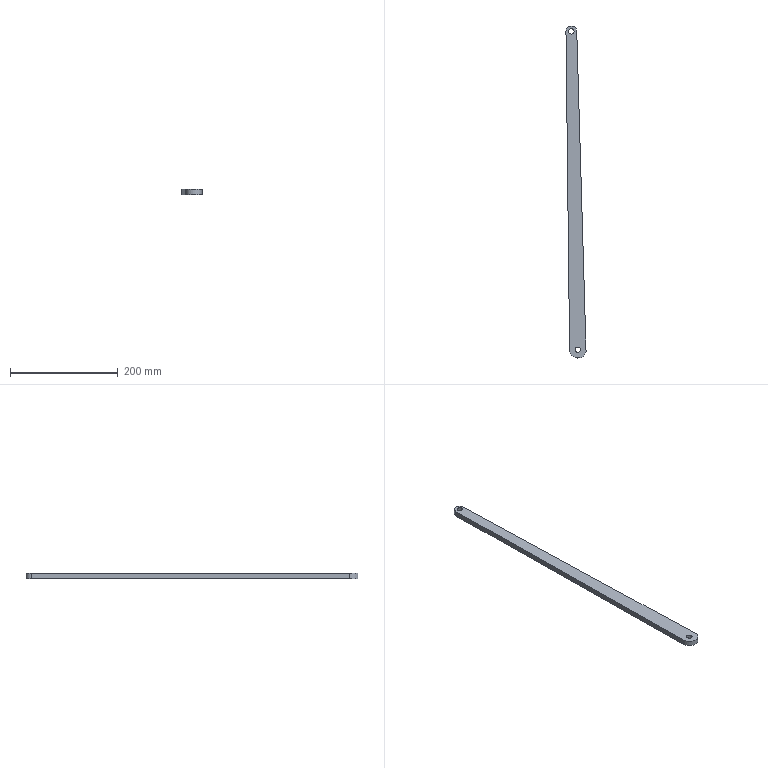Part | SolidWorks | features Extrusion 1 | 1 solid | 10 faces | box 37.197 x 615.099 x 10 mm | volume 152379 mm3 | cylinder 6 | plane 4 | commonest cylinder face diameters 10 x4 20 x1 30.679 x1
STEP:
#1=CARTESIAN_POINT('',(-4.803,1272.712,10.));
#2=VERTEX_POINT('',#1);
#3=CARTESIAN_POINT('',(5.197,1272.712,10.));
#4=VERTEX_POINT('',#3);
#5=CARTESIAN_POINT('',(0.1973,1272.712,10.));
#6=DIRECTION('',(0.,0.,1.));
#7=DIRECTION('',(1.,0.,0.));
#8=AXIS2_PLACEMENT_3D('',#5,#6,#7);
#9=CIRCLE('',#8,5.);
#10=EDGE_CURVE('',#2,#4,#9,.T.);
#11=ORIENTED_EDGE('',*,*,#10,.T.);
#12=CARTESIAN_POINT('',(5.197,1272.712,0.));
#13=VERTEX_POINT('',#12);
#14=CARTESIAN_POINT('',(5.197,1272.712,10.));
#15=DIRECTION('',(0.,0.,-1.));
#16=VECTOR('',#15,1000.);
#17=LINE('',#14,#16);
#18=EDGE_CURVE('',#4,#13,#17,.T.);
#19=ORIENTED_EDGE('',*,*,#18,.T.);
#20=CARTESIAN_POINT('',(-4.803,1272.712,0.));
#21=VERTEX_POINT('',#20);
#22=CARTESIAN_POINT('',(0.1973,1272.712,0.));
#23=DIRECTION('',(0.,0.,1.));
#24=DIRECTION('',(1.,0.,0.));
#25=AXIS2_PLACEMENT_3D('',#22,#23,#24);
#26=CIRCLE('',#25,5.);
#27=EDGE_CURVE('',#21,#13,#26,.T.);
#28=ORIENTED_EDGE('',*,*,#27,.F.);
#29=CARTESIAN_POINT('',(-4.803,1272.712,10.));
#30=DIRECTION('',(0.,0.,-1.));
#31=VECTOR('',#30,1000.);
#32=LINE('',#29,#31);
#33=EDGE_CURVE('',#2,#21,#32,.T.);
#34=ORIENTED_EDGE('',*,*,#33,.F.);
#35=EDGE_LOOP('',(#11,#19,#28,#34));
#36=FACE_OUTER_BOUND('',#35,.T.);
#37=CARTESIAN_POINT('',(0.1973,1272.712,10.));
#38=DIRECTION('',(0.,0.,-1.));
#39=DIRECTION('',(-1.,0.,0.));
#40=AXIS2_PLACEMENT_3D('',#37,#38,#39);
#41=CYLINDRICAL_SURFACE('',#40,5.);
#42=ADVANCED_FACE('',(#36),#41,.F.);
#43=CARTESIAN_POINT('',(7.243,682.953,10.));
#44=VERTEX_POINT('',#43);
#45=CARTESIAN_POINT('',(17.243,682.953,10.));
#46=VERTEX_POINT('',#45);
#47=CARTESIAN_POINT('',(12.243,682.953,10.));
#48=DIRECTION('',(0.,0.,1.));
#49=DIRECTION('',(1.,0.,0.));
#50=AXIS2_PLACEMENT_3D('',#47,#48,#49);
#51=CIRCLE('',#50,5.);
#52=EDGE_CURVE('',#44,#46,#51,.T.);
#53=ORIENTED_EDGE('',*,*,#52,.T.);
#54=CARTESIAN_POINT('',(17.243,682.953,0.));
#55=VERTEX_POINT('',#54);
#56=CARTESIAN_POINT('',(17.243,682.953,10.));
#57=DIRECTION('',(0.,0.,-1.));
#58=VECTOR('',#57,1000.);
#59=LINE('',#56,#58);
#60=EDGE_CURVE('',#46,#55,#59,.T.);
#61=ORIENTED_EDGE('',*,*,#60,.T.);
#62=CARTESIAN_POINT('',(7.243,682.953,0.));
#63=VERTEX_POINT('',#62);
#64=CARTESIAN_POINT('',(12.243,682.953,0.));
#65=DIRECTION('',(0.,0.,1.));
#66=DIRECTION('',(1.,0.,0.));
#67=AXIS2_PLACEMENT_3D('',#64,#65,#66);
#68=CIRCLE('',#67,5.);
#69=EDGE_CURVE('',#63,#55,#68,.T.);
#70=ORIENTED_EDGE('',*,*,#69,.F.);
#71=CARTESIAN_POINT('',(7.243,682.953,10.));
#72=DIRECTION('',(0.,0.,-1.));
#73=VECTOR('',#72,1000.);
#74=LINE('',#71,#73);
#75=EDGE_CURVE('',#44,#63,#74,.T.);
#76=ORIENTED_EDGE('',*,*,#75,.F.);
#77=EDGE_LOOP('',(#53,#61,#70,#76));
#78=FACE_OUTER_BOUND('',#77,.T.);
#79=CARTESIAN_POINT('',(12.243,682.953,10.));
#80=DIRECTION('',(0.,0.,-1.));
#81=DIRECTION('',(-1.,0.,0.));
#82=AXIS2_PLACEMENT_3D('',#79,#80,#81);
#83=CYLINDRICAL_SURFACE('',#82,5.);
#84=ADVANCED_FACE('',(#78),#83,.F.);
#85=CARTESIAN_POINT('',(-3.096,682.778,0.));
#86=VERTEX_POINT('',#85);
#87=CARTESIAN_POINT('',(-9.803,1272.712,0.));
#88=VERTEX_POINT('',#87);
#89=CARTESIAN_POINT('',(4.666,0.05305,0.));
#90=DIRECTION('',(-0.01137,0.9999,0.));
#91=VECTOR('',#90,1000.);
#92=LINE('',#89,#91);
#93=EDGE_CURVE('',#86,#88,#92,.T.);
#94=ORIENTED_EDGE('',*,*,#93,.F.);
#95=CARTESIAN_POINT('',(-3.096,682.778,10.));
#96=VERTEX_POINT('',#95);
#97=CARTESIAN_POINT('',(-3.096,682.778,10.));
#98=DIRECTION('',(0.,0.,-1.));
#99=VECTOR('',#98,1000.);
#100=LINE('',#97,#99);
#101=EDGE_CURVE('',#96,#86,#100,.T.);
#102=ORIENTED_EDGE('',*,*,#101,.F.);
#103=CARTESIAN_POINT('',(-9.803,1272.712,10.));
#104=VERTEX_POINT('',#103);
#105=CARTESIAN_POINT('',(4.666,0.05305,10.));
#106=DIRECTION('',(-0.01137,0.9999,0.));
#107=VECTOR('',#106,1000.);
#108=LINE('',#105,#107);
#109=EDGE_CURVE('',#96,#104,#108,.T.);
#110=ORIENTED_EDGE('',*,*,#109,.T.);
#111=CARTESIAN_POINT('',(-9.803,1272.712,10.));
#112=DIRECTION('',(0.,0.,-1.));
#113=VECTOR('',#112,1000.);
#114=LINE('',#111,#113);
#115=EDGE_CURVE('',#104,#88,#114,.T.);
#116=ORIENTED_EDGE('',*,*,#115,.T.);
#117=EDGE_LOOP('',(#94,#102,#110,#116));
#118=FACE_OUTER_BOUND('',#117,.T.);
#119=CARTESIAN_POINT('',(4.666,0.05305,10.));
#120=DIRECTION('',(-0.9999,-0.01137,0.));
#121=DIRECTION('',(0.01137,-0.9999,0.));
#122=AXIS2_PLACEMENT_3D('',#119,#120,#121);
#123=PLANE('',#122);
#124=ADVANCED_FACE('',(#118),#123,.T.);
#125=CARTESIAN_POINT('',(27.395,680.56,0.));
#126=VERTEX_POINT('',#125);
#127=CARTESIAN_POINT('',(12.243,682.953,0.));
#128=DIRECTION('',(0.,0.,1.));
#129=DIRECTION('',(1.,0.,0.));
#130=AXIS2_PLACEMENT_3D('',#127,#128,#129);
#131=CIRCLE('',#130,15.34);
#132=EDGE_CURVE('',#86,#126,#131,.T.);
#133=ORIENTED_EDGE('',*,*,#132,.T.);
#134=CARTESIAN_POINT('',(27.395,680.56,10.));
#135=VERTEX_POINT('',#134);
#136=CARTESIAN_POINT('',(27.395,680.56,10.));
#137=DIRECTION('',(0.,0.,-1.));
#138=VECTOR('',#137,1000.);
#139=LINE('',#136,#138);
#140=EDGE_CURVE('',#135,#126,#139,.T.);
#141=ORIENTED_EDGE('',*,*,#140,.F.);
#142=CARTESIAN_POINT('',(12.243,682.953,10.));
#143=DIRECTION('',(0.,0.,1.));
#144=DIRECTION('',(1.,0.,0.));
#145=AXIS2_PLACEMENT_3D('',#142,#143,#144);
#146=CIRCLE('',#145,15.34);
#147=EDGE_CURVE('',#96,#135,#146,.T.);
#148=ORIENTED_EDGE('',*,*,#147,.F.);
#149=ORIENTED_EDGE('',*,*,#101,.T.);
#150=EDGE_LOOP('',(#133,#141,#148,#149));
#151=FACE_OUTER_BOUND('',#150,.T.);
#152=CARTESIAN_POINT('',(12.243,682.953,10.));
#153=DIRECTION('',(0.,0.,-1.));
#154=DIRECTION('',(-1.,0.,0.));
#155=AXIS2_PLACEMENT_3D('',#152,#153,#154);
#156=CYLINDRICAL_SURFACE('',#155,15.34);
#157=ADVANCED_FACE('',(#151),#156,.T.);
#158=CARTESIAN_POINT('',(10.197,1272.712,0.));
#159=VERTEX_POINT('',#158);
#160=CARTESIAN_POINT('',(47.12,1.368,0.));
#161=DIRECTION('',(0.02903,-0.9996,0.));
#162=VECTOR('',#161,1000.);
#163=LINE('',#160,#162);
#164=EDGE_CURVE('',#159,#126,#163,.T.);
#165=ORIENTED_EDGE('',*,*,#164,.F.);
#166=CARTESIAN_POINT('',(10.197,1272.712,10.));
#167=VERTEX_POINT('',#166);
#168=CARTESIAN_POINT('',(10.197,1272.712,10.));
#169=DIRECTION('',(0.,0.,-1.));
#170=VECTOR('',#169,1000.);
#171=LINE('',#168,#170);
#172=EDGE_CURVE('',#167,#159,#171,.T.);
#173=ORIENTED_EDGE('',*,*,#172,.F.);
#174=CARTESIAN_POINT('',(47.12,1.368,10.));
#175=DIRECTION('',(0.02903,-0.9996,0.));
#176=VECTOR('',#175,1000.);
#177=LINE('',#174,#176);
#178=EDGE_CURVE('',#167,#135,#177,.T.);
#179=ORIENTED_EDGE('',*,*,#178,.T.);
#180=ORIENTED_EDGE('',*,*,#140,.T.);
#181=EDGE_LOOP('',(#165,#173,#179,#180));
#182=FACE_OUTER_BOUND('',#181,.T.);
#183=CARTESIAN_POINT('',(47.12,1.368,10.));
#184=DIRECTION('',(0.9996,0.02903,0.));
#185=DIRECTION('',(-0.02903,0.9996,0.));
#186=AXIS2_PLACEMENT_3D('',#183,#184,#185);
#187=PLANE('',#186);
#188=ADVANCED_FACE('',(#182),#187,.T.);
#189=ORIENTED_EDGE('',*,*,#60,.F.);
#190=CARTESIAN_POINT('',(12.243,682.953,10.));
#191=DIRECTION('',(0.,0.,1.));
#192=DIRECTION('',(1.,0.,0.));
#193=AXIS2_PLACEMENT_3D('',#190,#191,#192);
#194=CIRCLE('',#193,5.);
#195=EDGE_CURVE('',#46,#44,#194,.T.);
#196=ORIENTED_EDGE('',*,*,#195,.T.);
#197=ORIENTED_EDGE('',*,*,#75,.T.);
#198=CARTESIAN_POINT('',(12.243,682.953,0.));
#199=DIRECTION('',(0.,0.,1.));
#200=DIRECTION('',(1.,0.,0.));
#201=AXIS2_PLACEMENT_3D('',#198,#199,#200);
#202=CIRCLE('',#201,5.);
#203=EDGE_CURVE('',#55,#63,#202,.T.);
#204=ORIENTED_EDGE('',*,*,#203,.F.);
#205=EDGE_LOOP('',(#189,#196,#197,#204));
#206=FACE_OUTER_BOUND('',#205,.T.);
#207=CARTESIAN_POINT('',(12.243,682.953,10.));
#208=DIRECTION('',(0.,0.,-1.));
#209=DIRECTION('',(-1.,0.,0.));
#210=AXIS2_PLACEMENT_3D('',#207,#208,#209);
#211=CYLINDRICAL_SURFACE('',#210,5.);
#212=ADVANCED_FACE('',(#206),#211,.F.);
#213=ORIENTED_EDGE('',*,*,#18,.F.);
#214=CARTESIAN_POINT('',(0.1973,1272.712,10.));
#215=DIRECTION('',(0.,0.,1.));
#216=DIRECTION('',(1.,0.,0.));
#217=AXIS2_PLACEMENT_3D('',#214,#215,#216);
#218=CIRCLE('',#217,5.);
#219=EDGE_CURVE('',#4,#2,#218,.T.);
#220=ORIENTED_EDGE('',*,*,#219,.T.);
#221=ORIENTED_EDGE('',*,*,#33,.T.);
#222=CARTESIAN_POINT('',(0.1973,1272.712,0.));
#223=DIRECTION('',(0.,0.,1.));
#224=DIRECTION('',(1.,0.,0.));
#225=AXIS2_PLACEMENT_3D('',#222,#223,#224);
#226=CIRCLE('',#225,5.);
#227=EDGE_CURVE('',#13,#21,#226,.T.);
#228=ORIENTED_EDGE('',*,*,#227,.F.);
#229=EDGE_LOOP('',(#213,#220,#221,#228));
#230=FACE_OUTER_BOUND('',#229,.T.);
#231=CARTESIAN_POINT('',(0.1973,1272.712,10.));
#232=DIRECTION('',(0.,0.,-1.));
#233=DIRECTION('',(-1.,0.,0.));
#234=AXIS2_PLACEMENT_3D('',#231,#232,#233);
#235=CYLINDRICAL_SURFACE('',#234,5.);
#236=ADVANCED_FACE('',(#230),#235,.F.);
#237=CARTESIAN_POINT('',(0.1973,1272.712,0.));
#238=DIRECTION('',(0.,0.,1.));
#239=DIRECTION('',(1.,0.,0.));
#240=AXIS2_PLACEMENT_3D('',#237,#238,#239);
#241=CIRCLE('',#240,10.);
#242=EDGE_CURVE('',#159,#88,#241,.T.);
#243=ORIENTED_EDGE('',*,*,#242,.T.);
#244=ORIENTED_EDGE('',*,*,#115,.F.);
#245=CARTESIAN_POINT('',(0.1973,1272.712,10.));
#246=DIRECTION('',(0.,0.,1.));
#247=DIRECTION('',(1.,0.,0.));
#248=AXIS2_PLACEMENT_3D('',#245,#246,#247);
#249=CIRCLE('',#248,10.);
#250=EDGE_CURVE('',#167,#104,#249,.T.);
#251=ORIENTED_EDGE('',*,*,#250,.F.);
#252=ORIENTED_EDGE('',*,*,#172,.T.);
#253=EDGE_LOOP('',(#243,#244,#251,#252));
#254=FACE_OUTER_BOUND('',#253,.T.);
#255=CARTESIAN_POINT('',(0.1973,1272.712,10.));
#256=DIRECTION('',(0.,0.,-1.));
#257=DIRECTION('',(-1.,0.,0.));
#258=AXIS2_PLACEMENT_3D('',#255,#256,#257);
#259=CYLINDRICAL_SURFACE('',#258,10.);
#260=ADVANCED_FACE('',(#254),#259,.T.);
#261=ORIENTED_EDGE('',*,*,#10,.F.);
#262=ORIENTED_EDGE('',*,*,#219,.F.);
#263=EDGE_LOOP('',(#261,#262));
#264=FACE_BOUND('',#263,.T.);
#265=ORIENTED_EDGE('',*,*,#52,.F.);
#266=ORIENTED_EDGE('',*,*,#195,.F.);
#267=EDGE_LOOP('',(#265,#266));
#268=FACE_BOUND('',#267,.T.);
#269=ORIENTED_EDGE('',*,*,#109,.F.);
#270=ORIENTED_EDGE('',*,*,#147,.T.);
#271=ORIENTED_EDGE('',*,*,#178,.F.);
#272=ORIENTED_EDGE('',*,*,#250,.T.);
#273=EDGE_LOOP('',(#269,#270,#271,#272));
#274=FACE_OUTER_BOUND('',#273,.T.);
#275=CARTESIAN_POINT('',(0.,0.,10.));
#276=DIRECTION('',(0.,0.,1.));
#277=DIRECTION('',(1.,0.,0.));
#278=AXIS2_PLACEMENT_3D('',#275,#276,#277);
#279=PLANE('',#278);
#280=ADVANCED_FACE('',(#264,#268,#274),#279,.T.);
#281=ORIENTED_EDGE('',*,*,#27,.T.);
#282=ORIENTED_EDGE('',*,*,#227,.T.);
#283=EDGE_LOOP('',(#281,#282));
#284=FACE_BOUND('',#283,.T.);
#285=ORIENTED_EDGE('',*,*,#69,.T.);
#286=ORIENTED_EDGE('',*,*,#203,.T.);
#287=EDGE_LOOP('',(#285,#286));
#288=FACE_BOUND('',#287,.T.);
#289=ORIENTED_EDGE('',*,*,#93,.T.);
#290=ORIENTED_EDGE('',*,*,#242,.F.);
#291=ORIENTED_EDGE('',*,*,#164,.T.);
#292=ORIENTED_EDGE('',*,*,#132,.F.);
#293=EDGE_LOOP('',(#289,#290,#291,#292));
#294=FACE_OUTER_BOUND('',#293,.T.);
#295=CARTESIAN_POINT('',(0.,0.,0.));
#296=DIRECTION('',(0.,0.,1.));
#297=DIRECTION('',(1.,0.,0.));
#298=AXIS2_PLACEMENT_3D('',#295,#296,#297);
#299=PLANE('',#298);
#300=ADVANCED_FACE('',(#284,#288,#294),#299,.F.);
#301=CLOSED_SHELL('',(#42,#84,#124,#157,#188,#212,#236,#260,#280,#300));
#302=MANIFOLD_SOLID_BREP('',#301);
#303=CARTESIAN_POINT('',(0.,0.,0.));
#304=DIRECTION('',(0.,0.,1.));
#305=DIRECTION('',(1.,0.,0.));
#306=AXIS2_PLACEMENT_3D('',#303,#304,#305);
#307=(LENGTH_UNIT()NAMED_UNIT(*)SI_UNIT(.MILLI.,.METRE.));
#308=UNCERTAINTY_MEASURE_WITH_UNIT(LENGTH_MEASURE(0.00001),#307,'','');
#309=(NAMED_UNIT(*)PLANE_ANGLE_UNIT()SI_UNIT($,.RADIAN.));
#310=(NAMED_UNIT(*)SI_UNIT($,.STERADIAN.)SOLID_ANGLE_UNIT());
#311=(GEOMETRIC_REPRESENTATION_CONTEXT(3)GLOBAL_UNCERTAINTY_ASSIGNED_CONTEXT((#308))GLOBAL_UNIT_ASSIGNED_CONTEXT((#307,#309,#310))REPRESENTATION_CONTEXT('',''));
#312=ADVANCED_BREP_SHAPE_REPRESENTATION('',(#302,#306),#311);